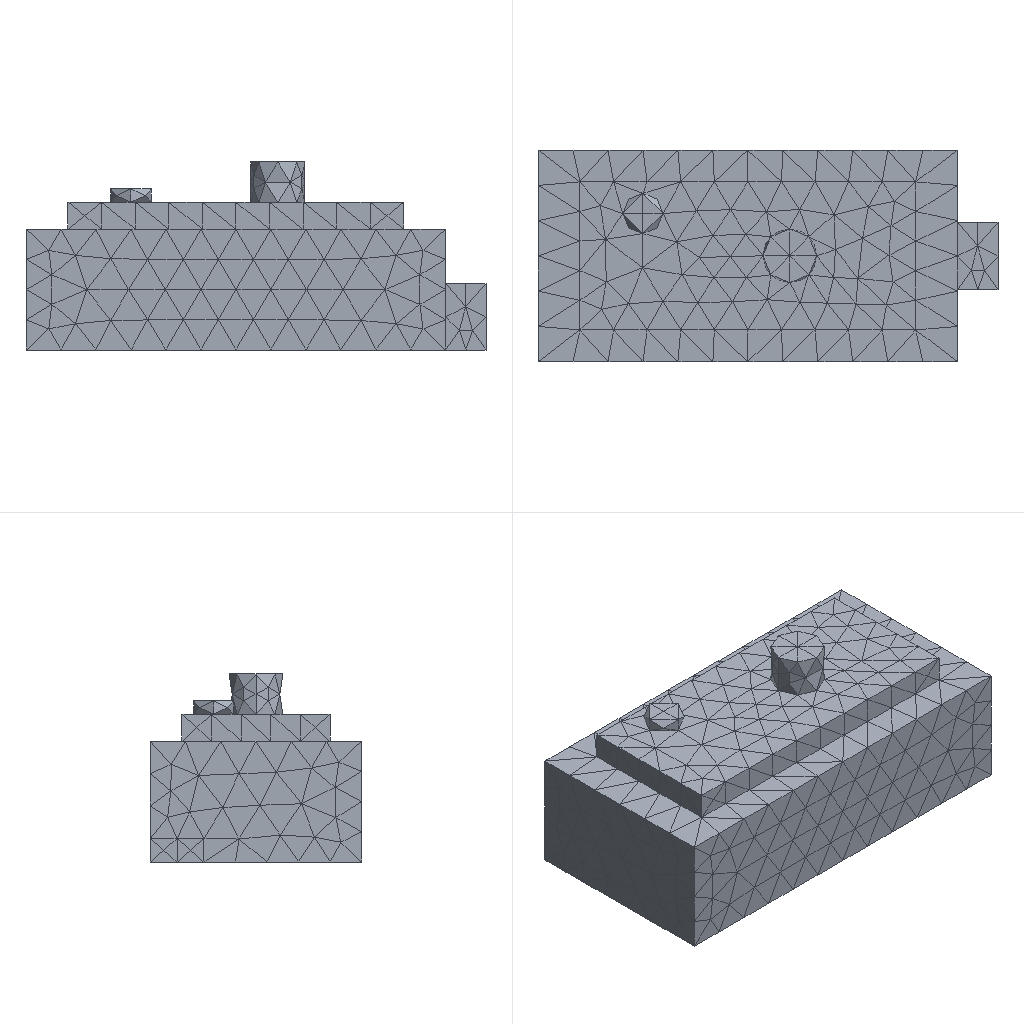Simulation study | ansys mapdl
Set-up summary:
category,name,step,type,value,unit,region
solver,ansys_mapdl
units,mm-N-s-tonne (MPa),,inferred,E=210000 density=
analysis,model,,static
mesh,nodes,,,4651
mesh,elements,,,2767
element_type,SOLID187,,,2767
material,mat 1,,E,210000
material,mat 1,,nu,0.3
load,,model,body load temp,,,all
load,,model,force,"1000 [dir=(0, 0, -1) n=218]",,node list
bc,,model,fixed,"[dofs=UX,UY,UZ n=4850]",,node list
Ansys APDL input file, long lists of numbers shortened:
/COM,ANSYS RELEASE 2026 R1           BUILD 26.1      UP20260202       09:10:49
/PREP7
/NOPR
/TITLE,2
ANTYPE, 0
*IF,_CDRDOFF,EQ,1,THEN     !if solid model was read in
_CDRDOFF=             !reset flag, numoffs already performed
*ELSE              !offset database for the following FE model
NUMOFF,NODE,     4651
NUMOFF,ELEM,     2767
NUMOFF,MAT ,        1
NUMOFF,TYPE,        1
*ENDIF
*SET,_RETURN ,  0.
*SET,_STATUS ,  0.
*SET,_UIQR   ,  218.
*SET,__FLOATPARAMETER__,  4651.
DOF,DELETE
ETBLOCK,        1,        1
(2i9,19a9)
        1      187        0        0        0        0        0        0        0        0        0        0        0        0        0        0        0        0        0        0        0
       -1
NBLOCK,6,SOLID,      4651,      4651
(3i9,6e21.13e3)
        1        0        0-4.6500000000000E+001 3.1500000000000E+001 7.0000000000000E+000
! (4650 more lines like these left out)
N,UNBL,LOC,       -1,
EBLOCK,19,SOLID,      2767,      2767
(19i10)
         1         1         1         1         0         0         0         0        10         0         1      1831      1832      1833      1834      2086      2087      2088      2089
! (5533 more lines like these left out)
        -1
MPTEMP,UNBL, 1, 1,  0.    ,
MPDATA,UNBL, 1,EX  ,       1, 1,  210000.000    ,
MPTEMP,UNBL, 1, 1,  0.    ,
MPDATA,UNBL, 1,NUXY,       1, 1, 0.3    ,
MPTEMP,UNBL, 1, 1,  0.    ,
MPDATA,UNBL, 1,PRXY,       1, 1, 0.3    ,
EXTOPT,ATTR,      0,      0,      0
EXTOPT,ESIZE,  0,  0.
EXTOPT,ACLEAR,      0
TREF,  0.
IRLF,  0
BFUNIF,TEMP,_TINY
ACEL,  0.    ,  0.    ,  0.
OMEGA,  0.    ,  0.    ,  0.
DOMEGA,  0.    ,  0.    ,  0.
CGLOC,  0.    ,  0.    ,  0.
CGOMEGA,  0.    ,  0.    ,  0.
DCGOMG,  0.    ,  0.    ,  0.
KUSE,     0
TIME,  0.
ALPHAD,  0.
BETAD,  0.
DMPRAT,  0.
DMPSTR,  0.
CRPLIM, 0.1    ,   0
CRPLIM,  0.    ,   1
NCNV,     0, 1.000000000E+12,     0,  0.    ,  0.
NEQIT,     0
ERESX,DEFA
DBLOCK,      4850
(i9,a6,2(pg16.9))
        1  UX    0.00000000      0.00000000
! (4849 more lines like these left out)
       -1
FBLOCK,       218
(i9,a6,2(pg16.9))
      914  FZ   -4.58715596      0.00000000
! (217 more lines like these left out)
       -1
/GO
FINISH
Results summary:
result,analysis_type_db,,,static,unstated
result,n_sets,,,1,unstated
result,load_steps[0].set,load_step=1,,1,unstated
result,load_steps[0].substep,load_step=1,,1,unstated
result,load_steps[0].time,load_step=1,,1,unstated
result,load_steps[0].freq,load_step=1,,1,unstated
result,load_steps[0].max_usum,load_step=1,,0.0003553,unstated
result,load_steps[0].max_seqv,load_step=1,,4.201,unstated
result,load_steps[0].reaction_sum.FX,load_step=1,,2.06981e-11,unstated
result,load_steps[0].reaction_sum.FY,load_step=1,,-4.02345e-12,unstated
result,load_steps[0].reaction_sum.FZ,load_step=1,,1000,unstated
result,load_steps[0].reaction_sum.MX,load_step=1,,0,unstated
result,load_steps[0].reaction_sum.MY,load_step=1,,0,unstated
result,load_steps[0].reaction_sum.MZ,load_step=1,,0,unstated
result,convergence,,,results present for all listed sets,unstated